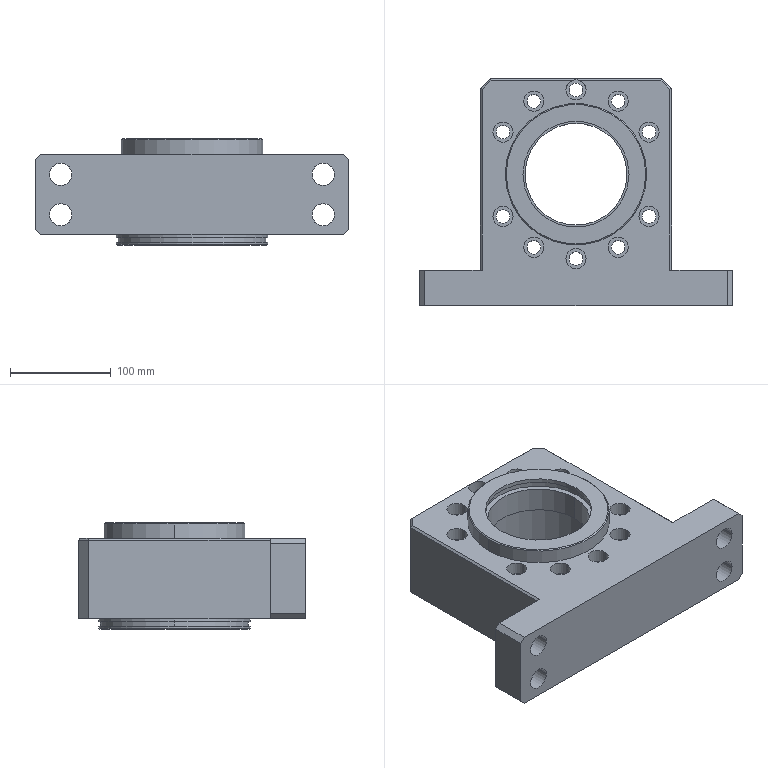Part | SolidWorks | features ICE 16, Chamfer 5, HoleWzd 4, CirPattern 2, MirrorPattern 2, Extrusion 1, Fillet 1 | 1 solid | 160 faces | box 310 x 225 x 105 mm | volume 2847802 mm3 | cylinder 88 | plane 52 | cone 20 | commonest cylinder face diameters 13.5 x20 20 x20 8.5 x16 22 x8 30 x4 120 x4